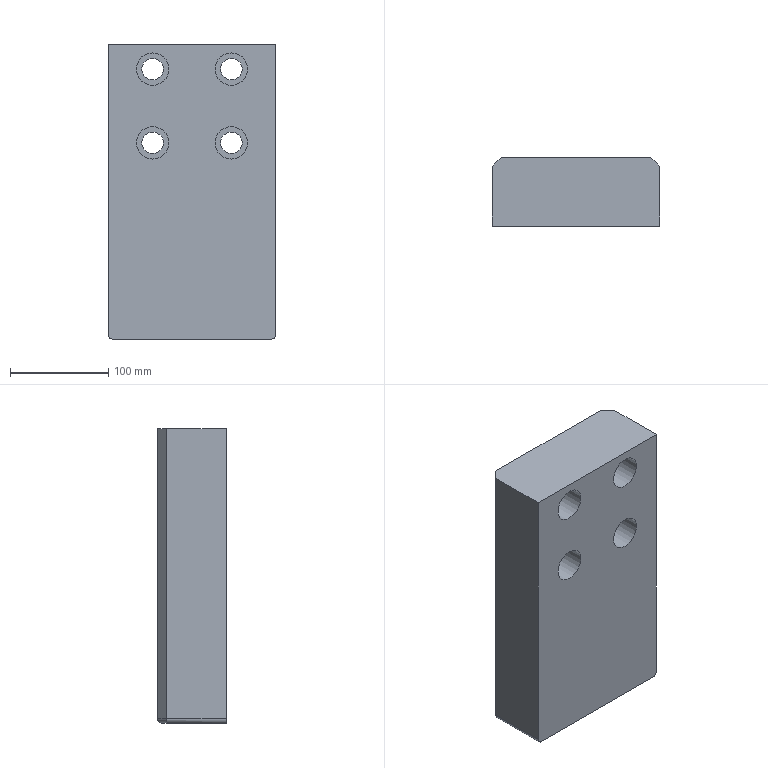Part | STEP file | 220_id82_x_t | 1 solid | 27 faces | box 170 x 70 x 300 mm | volume 3373975 mm3 | cylinder 14 | plane 12 | cone 1 | commonest cylinder face diameters 10 x5 22 x4 33 x4 14 x1